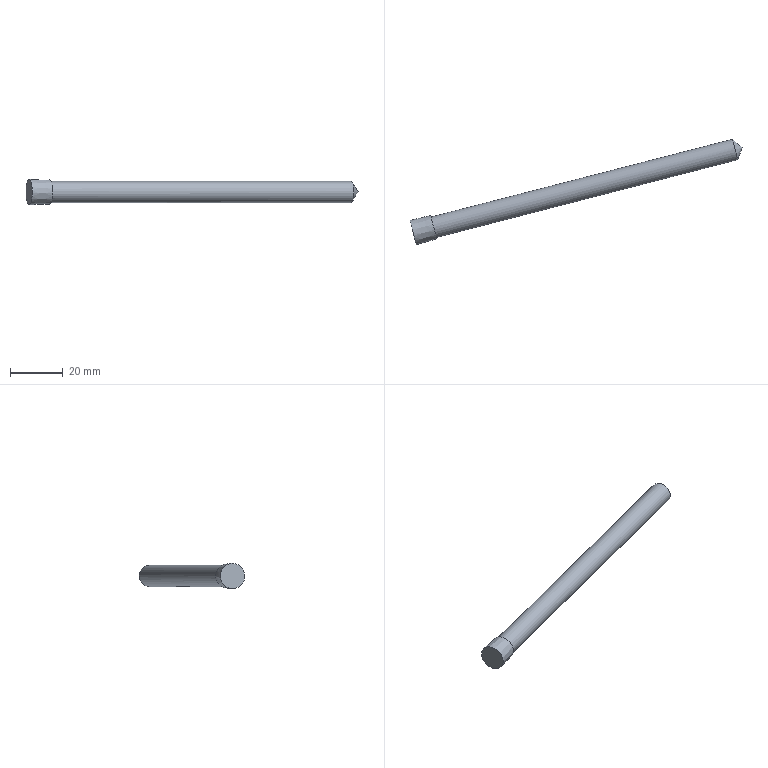Part | STEP file | 车灯-后视镜_id546_x_t | 1 solid | 5 faces | box 125.408 x 39.857 x 9.556 mm | volume 6500 mm3 | plane 2 | cone 2 | cylinder 1 | commonest cylinder face diameters 8 x1
STEP:
#1=CARTESIAN_POINT('',(-248.674,33.419,14.714));
#2=VERTEX_POINT('',#1);
#3=CARTESIAN_POINT('',(-247.675,29.546,14.714));
#4=DIRECTION('',(-0.9683,-0.2497,0.));
#5=DIRECTION('',(-0.2497,0.9683,0.));
#6=AXIS2_PLACEMENT_3D('',#3,#4,#5);
#7=CIRCLE('',#6,4.);
#8=EDGE_CURVE('',#2,#2,#7,.T.);
#9=ORIENTED_EDGE('',*,*,#8,.T.);
#10=EDGE_LOOP('',(#9));
#11=FACE_BOUND('',#10,.T.);
#12=CARTESIAN_POINT('',(-247.675,29.546,10.179));
#13=VERTEX_POINT('',#12);
#14=CARTESIAN_POINT('',(-247.675,29.546,14.714));
#15=DIRECTION('',(0.9683,0.2497,0.));
#16=DIRECTION('',(0.,0.,-1.));
#17=AXIS2_PLACEMENT_3D('',#14,#15,#16);
#18=CIRCLE('',#17,4.535);
#19=EDGE_CURVE('',#13,#13,#18,.T.);
#20=ORIENTED_EDGE('',*,*,#19,.T.);
#21=EDGE_LOOP('',(#20));
#22=FACE_BOUND('',#21,.T.);
#23=CARTESIAN_POINT('',(-247.675,29.546,14.714));
#24=DIRECTION('',(0.9683,0.2497,0.));
#25=DIRECTION('',(0.,0.,1.));
#26=AXIS2_PLACEMENT_3D('',#23,#24,#25);
#27=PLANE('',#26);
#28=ADVANCED_FACE('',(#11,#22),#27,.T.);
#29=CARTESIAN_POINT('',(-255.124,26.393,10.088));
#30=VERTEX_POINT('',#29);
#31=CARTESIAN_POINT('',(-255.422,27.548,14.714));
#32=DIRECTION('',(-0.9683,-0.2497,0.));
#33=DIRECTION('',(0.06235,-0.2418,-0.9683));
#34=AXIS2_PLACEMENT_3D('',#31,#32,#33);
#35=CIRCLE('',#34,4.778);
#36=EDGE_CURVE('',#30,#30,#35,.T.);
#37=ORIENTED_EDGE('',*,*,#36,.F.);
#38=EDGE_LOOP('',(#37));
#39=FACE_BOUND('',#38,.T.);
#40=ORIENTED_EDGE('',*,*,#19,.F.);
#41=EDGE_LOOP('',(#40));
#42=FACE_BOUND('',#41,.T.);
#43=CARTESIAN_POINT('',(-247.675,29.546,14.714));
#44=DIRECTION('',(-0.9683,-0.2497,0.));
#45=DIRECTION('',(0.,0.,-1.));
#46=AXIS2_PLACEMENT_3D('',#43,#44,#45);
#47=CONICAL_SURFACE('',#46,4.535,1.738);
#48=ADVANCED_FACE('',(#39,#42),#47,.T.);
#49=ORIENTED_EDGE('',*,*,#8,.F.);
#50=EDGE_LOOP('',(#49));
#51=FACE_BOUND('',#50,.T.);
#52=CARTESIAN_POINT('',(-134.069,59.872,18.588));
#53=VERTEX_POINT('',#52);
#54=CARTESIAN_POINT('',(-133.82,58.905,14.714));
#55=DIRECTION('',(0.9683,0.2497,0.));
#56=DIRECTION('',(-0.06235,0.2418,0.9683));
#57=AXIS2_PLACEMENT_3D('',#54,#55,#56);
#58=CIRCLE('',#57,4.);
#59=EDGE_CURVE('',#53,#53,#58,.T.);
#60=ORIENTED_EDGE('',*,*,#59,.F.);
#61=EDGE_LOOP('',(#60));
#62=FACE_BOUND('',#61,.T.);
#63=CARTESIAN_POINT('',(-215.643,37.806,14.714));
#64=DIRECTION('',(0.9683,0.2497,0.));
#65=DIRECTION('',(0.,0.,1.));
#66=AXIS2_PLACEMENT_3D('',#63,#64,#65);
#67=CYLINDRICAL_SURFACE('',#66,4.);
#68=ADVANCED_FACE('',(#51,#62),#67,.T.);
#69=ORIENTED_EDGE('',*,*,#59,.T.);
#70=EDGE_LOOP('',(#69));
#71=FACE_BOUND('',#70,.T.);
#72=CARTESIAN_POINT('',(-131.207,59.579,14.714));
#73=VERTEX_POINT('',#72);
#74=VERTEX_LOOP('',#73);
#75=FACE_BOUND('',#74,.T.);
#76=CARTESIAN_POINT('',(-131.207,59.579,14.714));
#77=DIRECTION('',(-0.9683,-0.2497,0.));
#78=DIRECTION('',(0.,0.,1.));
#79=AXIS2_PLACEMENT_3D('',#76,#77,#78);
#80=CONICAL_SURFACE('',#79,0.,56.);
#81=ADVANCED_FACE('',(#71,#75),#80,.T.);
#82=ORIENTED_EDGE('',*,*,#36,.T.);
#83=EDGE_LOOP('',(#82));
#84=FACE_OUTER_BOUND('',#83,.T.);
#85=CARTESIAN_POINT('',(-255.422,27.548,14.714));
#86=DIRECTION('',(0.9683,0.2497,0.));
#87=DIRECTION('',(0.,0.,-1.));
#88=AXIS2_PLACEMENT_3D('',#85,#86,#87);
#89=PLANE('',#88);
#90=ADVANCED_FACE('',(#84),#89,.F.);
#91=CLOSED_SHELL('',(#28,#48,#68,#81,#90));
#92=MANIFOLD_SOLID_BREP('',#91);
#93=(LENGTH_UNIT()NAMED_UNIT(*)SI_UNIT(.MILLI.,.METRE.));
#94=UNCERTAINTY_MEASURE_WITH_UNIT(LENGTH_MEASURE(0.00002),#93,'','');
#95=(NAMED_UNIT(*)PLANE_ANGLE_UNIT()SI_UNIT($,.RADIAN.));
#96=PLANE_ANGLE_MEASURE_WITH_UNIT(PLANE_ANGLE_MEASURE(0.01745),#95);
#97=DIMENSIONAL_EXPONENTS(0.,0.,0.,0.,0.,0.,0.);
#98=(CONVERSION_BASED_UNIT('DEGREE',#96)NAMED_UNIT(#97)PLANE_ANGLE_UNIT());
#99=(NAMED_UNIT(*)SI_UNIT($,.STERADIAN.)SOLID_ANGLE_UNIT());
#100=(GEOMETRIC_REPRESENTATION_CONTEXT(3)GLOBAL_UNCERTAINTY_ASSIGNED_CONTEXT((#94))GLOBAL_UNIT_ASSIGNED_CONTEXT((#93,#98,#99))REPRESENTATION_CONTEXT('',''));
#101=ADVANCED_BREP_SHAPE_REPRESENTATION('',(#92),#100);